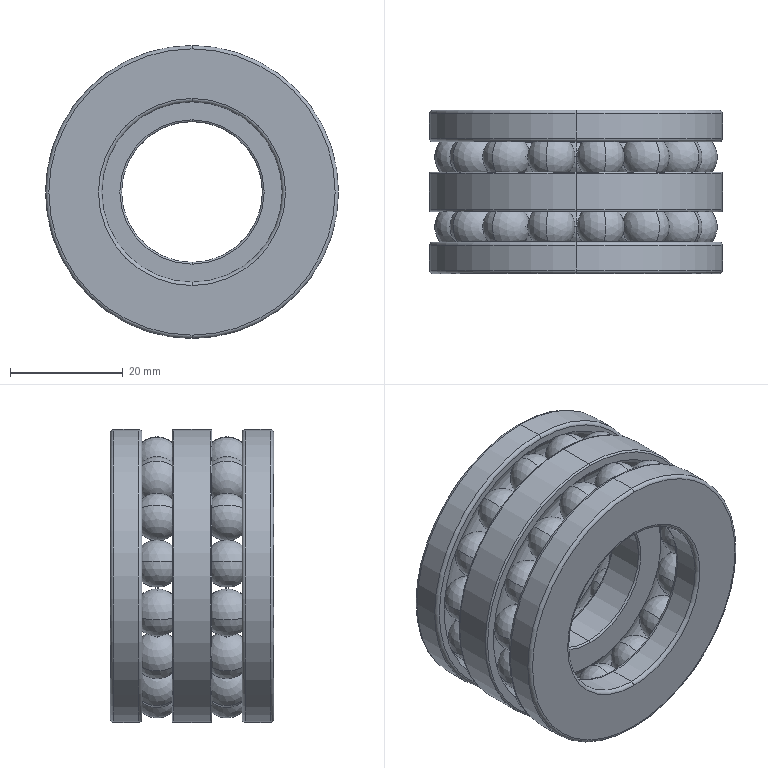Part | SolidWorks | features Revolution 2, CirPattern 1 | 33 solids | 114 faces | box 52 x 29 x 52 mm | volume 31888 mm3 | sphere 60 | torus 32 | cylinder 12 | plane 10 | commonest cylinder face diameters 52 x6 32 x4 25 x2